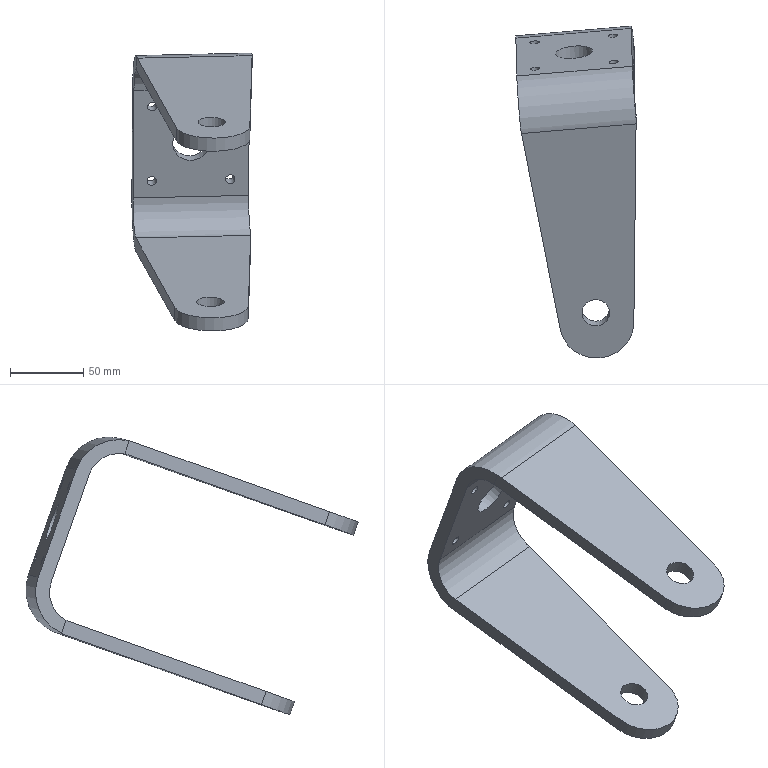Part | NX | features solid 2 | 1 solid | 25 faces | box 82.324 x 227.523 x 190.251 mm | volume 304271 mm3 | cylinder 13 | plane 12 | commonest cylinder face diameters 6.35 x4 19 x2 42.95 x2 50.8 x2 62 x2 25.4 x1
STEP:
#1=CARTESIAN_POINT('',(180.018,413.948,712.362));
#2=VERTEX_POINT('',#1);
#3=CARTESIAN_POINT('',(179.425,439.961,638.776));
#4=VERTEX_POINT('',#3);
#5=CARTESIAN_POINT('',(180.016,414.039,712.102));
#6=DIRECTION('',(0.007596,-0.3333,0.9428));
#7=VECTOR('',#6,1000.);
#8=LINE('',#5,#7);
#9=EDGE_CURVE('',#2,#4,#8,.F.);
#10=ORIENTED_EDGE('',*,*,#9,.T.);
#11=CARTESIAN_POINT('',(100.353,433.263,637.046));
#12=VERTEX_POINT('',#11);
#13=CARTESIAN_POINT('',(100.353,433.263,637.046));
#14=DIRECTION('',(0.9962,0.08438,0.0218));
#15=VECTOR('',#14,1000.);
#16=LINE('',#13,#15);
#17=EDGE_CURVE('',#4,#12,#16,.F.);
#18=ORIENTED_EDGE('',*,*,#17,.T.);
#19=CARTESIAN_POINT('',(100.945,407.25,710.631));
#20=VERTEX_POINT('',#19);
#21=CARTESIAN_POINT('',(100.354,433.179,637.281));
#22=DIRECTION('',(0.007596,-0.3333,0.9428));
#23=VECTOR('',#22,1000.);
#24=LINE('',#21,#23);
#25=EDGE_CURVE('',#12,#20,#24,.T.);
#26=ORIENTED_EDGE('',*,*,#25,.T.);
#27=CARTESIAN_POINT('',(100.945,407.25,710.631));
#28=DIRECTION('',(0.9962,0.08438,0.0218));
#29=VECTOR('',#28,1000.);
#30=LINE('',#27,#29);
#31=EDGE_CURVE('',#20,#2,#30,.T.);
#32=ORIENTED_EDGE('',*,*,#31,.T.);
#33=EDGE_LOOP('',(#10,#18,#26,#32));
#34=FACE_BOUND('',#33,.T.);
#35=CARTESIAN_POINT('',(166.841,435.935,646.855));
#36=VERTEX_POINT('',#35);
#37=CARTESIAN_POINT('',(166.865,434.877,649.848));
#38=DIRECTION('',(-0.08682,0.939,0.3327));
#39=DIRECTION('',(-0.007596,0.3333,-0.9428));
#40=AXIS2_PLACEMENT_3D('',#37,#38,#39);
#41=CIRCLE('',#40,3.175);
#42=EDGE_CURVE('',#36,#36,#41,.T.);
#43=ORIENTED_EDGE('',*,*,#42,.F.);
#44=EDGE_LOOP('',(#43));
#45=FACE_BOUND('',#44,.T.);
#46=CARTESIAN_POINT('',(113.482,413.391,696.565));
#47=VERTEX_POINT('',#46);
#48=CARTESIAN_POINT('',(113.506,412.333,699.559));
#49=DIRECTION('',(-0.08682,0.939,0.3327));
#50=DIRECTION('',(-0.007596,0.3333,-0.9428));
#51=AXIS2_PLACEMENT_3D('',#48,#49,#50);
#52=CIRCLE('',#51,3.175);
#53=EDGE_CURVE('',#47,#47,#52,.T.);
#54=ORIENTED_EDGE('',*,*,#53,.F.);
#55=EDGE_LOOP('',(#54));
#56=FACE_BOUND('',#55,.T.);
#57=CARTESIAN_POINT('',(167.251,417.946,697.742));
#58=VERTEX_POINT('',#57);
#59=CARTESIAN_POINT('',(167.275,416.888,700.736));
#60=DIRECTION('',(-0.08682,0.939,0.3327));
#61=DIRECTION('',(-0.007596,0.3333,-0.9428));
#62=AXIS2_PLACEMENT_3D('',#59,#60,#61);
#63=CIRCLE('',#62,3.175);
#64=EDGE_CURVE('',#58,#58,#63,.T.);
#65=ORIENTED_EDGE('',*,*,#64,.F.);
#66=EDGE_LOOP('',(#65));
#67=FACE_BOUND('',#66,.T.);
#68=CARTESIAN_POINT('',(140.089,427.838,662.73));
#69=VERTEX_POINT('',#68);
#70=CARTESIAN_POINT('',(140.185,423.605,674.704));
#71=DIRECTION('',(-0.08682,0.939,0.3327));
#72=DIRECTION('',(-0.007596,0.3333,-0.9428));
#73=AXIS2_PLACEMENT_3D('',#70,#71,#72);
#74=CIRCLE('',#73,12.7);
#75=EDGE_CURVE('',#69,#69,#74,.T.);
#76=ORIENTED_EDGE('',*,*,#75,.F.);
#77=EDGE_LOOP('',(#76));
#78=FACE_BOUND('',#77,.T.);
#79=CARTESIAN_POINT('',(113.072,431.381,645.678));
#80=VERTEX_POINT('',#79);
#81=CARTESIAN_POINT('',(113.096,430.322,648.672));
#82=DIRECTION('',(0.08682,-0.939,-0.3327));
#83=DIRECTION('',(-0.007596,0.3333,-0.9428));
#84=AXIS2_PLACEMENT_3D('',#81,#82,#83);
#85=CIRCLE('',#84,3.175);
#86=EDGE_CURVE('',#80,#80,#85,.T.);
#87=ORIENTED_EDGE('',*,*,#86,.T.);
#88=EDGE_LOOP('',(#87));
#89=FACE_BOUND('',#88,.T.);
#90=CARTESIAN_POINT('',(100.943,407.341,710.372));
#91=DIRECTION('',(-0.08682,0.939,0.3327));
#92=DIRECTION('',(0.9962,0.08438,0.0218));
#93=AXIS2_PLACEMENT_3D('',#90,#91,#92);
#94=PLANE('',#93);
#95=ADVANCED_FACE('',(#34,#45,#56,#67,#78,#89),#94,.T.);
#96=CARTESIAN_POINT('',(101.18,424.318,633.877));
#97=VERTEX_POINT('',#96);
#98=CARTESIAN_POINT('',(101.772,398.305,707.462));
#99=VERTEX_POINT('',#98);
#100=CARTESIAN_POINT('',(101.77,398.397,707.203));
#101=DIRECTION('',(0.007596,-0.3333,0.9428));
#102=VECTOR('',#101,1000.);
#103=LINE('',#100,#102);
#104=EDGE_CURVE('',#97,#99,#103,.T.);
#105=ORIENTED_EDGE('',*,*,#104,.F.);
#106=CARTESIAN_POINT('',(180.252,431.016,635.608));
#107=VERTEX_POINT('',#106);
#108=CARTESIAN_POINT('',(180.252,431.016,635.608));
#109=DIRECTION('',(0.9962,0.08438,0.0218));
#110=VECTOR('',#109,1000.);
#111=LINE('',#108,#110);
#112=EDGE_CURVE('',#97,#107,#111,.T.);
#113=ORIENTED_EDGE('',*,*,#112,.T.);
#114=CARTESIAN_POINT('',(180.845,405.003,709.193));
#115=VERTEX_POINT('',#114);
#116=CARTESIAN_POINT('',(180.843,405.095,708.934));
#117=DIRECTION('',(0.007596,-0.3333,0.9428));
#118=VECTOR('',#117,1000.);
#119=LINE('',#116,#118);
#120=EDGE_CURVE('',#115,#107,#119,.F.);
#121=ORIENTED_EDGE('',*,*,#120,.F.);
#122=CARTESIAN_POINT('',(101.772,398.305,707.462));
#123=DIRECTION('',(0.9962,0.08438,0.0218));
#124=VECTOR('',#123,1000.);
#125=LINE('',#122,#124);
#126=EDGE_CURVE('',#115,#99,#125,.F.);
#127=ORIENTED_EDGE('',*,*,#126,.T.);
#128=EDGE_LOOP('',(#105,#113,#121,#127));
#129=FACE_BOUND('',#128,.T.);
#130=CARTESIAN_POINT('',(167.692,424.873,649.673));
#131=VERTEX_POINT('',#130);
#132=CARTESIAN_POINT('',(167.692,425.933,646.68));
#133=DIRECTION('',(-0.08682,0.939,0.3327));
#134=DIRECTION('',(0.,-0.3339,0.9426));
#135=AXIS2_PLACEMENT_3D('',#132,#133,#134);
#136=CIRCLE('',#135,3.175);
#137=EDGE_CURVE('',#131,#131,#136,.T.);
#138=ORIENTED_EDGE('',*,*,#137,.T.);
#139=EDGE_LOOP('',(#138));
#140=FACE_BOUND('',#139,.T.);
#141=CARTESIAN_POINT('',(114.333,402.329,699.383));
#142=VERTEX_POINT('',#141);
#143=CARTESIAN_POINT('',(114.333,403.389,696.39));
#144=DIRECTION('',(-0.08682,0.939,0.3327));
#145=DIRECTION('',(0.,-0.3339,0.9426));
#146=AXIS2_PLACEMENT_3D('',#143,#144,#145);
#147=CIRCLE('',#146,3.175);
#148=EDGE_CURVE('',#142,#142,#147,.T.);
#149=ORIENTED_EDGE('',*,*,#148,.T.);
#150=EDGE_LOOP('',(#149));
#151=FACE_BOUND('',#150,.T.);
#152=CARTESIAN_POINT('',(168.102,406.883,700.56));
#153=VERTEX_POINT('',#152);
#154=CARTESIAN_POINT('',(168.102,407.944,697.567));
#155=DIRECTION('',(-0.08682,0.939,0.3327));
#156=DIRECTION('',(0.,-0.3339,0.9426));
#157=AXIS2_PLACEMENT_3D('',#154,#155,#156);
#158=CIRCLE('',#157,3.175);
#159=EDGE_CURVE('',#153,#153,#158,.T.);
#160=ORIENTED_EDGE('',*,*,#159,.T.);
#161=EDGE_LOOP('',(#160));
#162=FACE_BOUND('',#161,.T.);
#163=CARTESIAN_POINT('',(141.012,410.42,683.506));
#164=VERTEX_POINT('',#163);
#165=CARTESIAN_POINT('',(141.012,414.661,671.535));
#166=DIRECTION('',(-0.08682,0.939,0.3327));
#167=DIRECTION('',(0.,-0.3339,0.9426));
#168=AXIS2_PLACEMENT_3D('',#165,#166,#167);
#169=CIRCLE('',#168,12.7);
#170=EDGE_CURVE('',#164,#164,#169,.T.);
#171=ORIENTED_EDGE('',*,*,#170,.T.);
#172=EDGE_LOOP('',(#171));
#173=FACE_BOUND('',#172,.T.);
#174=CARTESIAN_POINT('',(113.923,420.318,648.496));
#175=VERTEX_POINT('',#174);
#176=CARTESIAN_POINT('',(113.923,421.378,645.503));
#177=DIRECTION('',(-0.08682,0.939,0.3327));
#178=DIRECTION('',(0.,-0.3339,0.9426));
#179=AXIS2_PLACEMENT_3D('',#176,#177,#178);
#180=CIRCLE('',#179,3.175);
#181=EDGE_CURVE('',#175,#175,#180,.F.);
#182=ORIENTED_EDGE('',*,*,#181,.F.);
#183=EDGE_LOOP('',(#182));
#184=FACE_BOUND('',#183,.T.);
#185=CARTESIAN_POINT('',(101.77,398.397,707.203));
#186=DIRECTION('',(-0.08682,0.939,0.3327));
#187=DIRECTION('',(0.9962,0.08438,0.0218));
#188=AXIS2_PLACEMENT_3D('',#185,#186,#187);
#189=PLANE('',#188);
#190=ADVANCED_FACE('',(#129,#140,#151,#162,#173,#184),#189,.F.);
#191=ORIENTED_EDGE('',*,*,#25,.F.);
#192=CARTESIAN_POINT('',(102.532,417.433,598.727));
#193=VERTEX_POINT('',#192);
#194=CARTESIAN_POINT('',(103.044,404.153,626.733));
#195=DIRECTION('',(-0.9962,-0.08438,-0.0218));
#196=DIRECTION('',(0.0844,-0.9964,0.));
#197=AXIS2_PLACEMENT_3D('',#194,#195,#196);
#198=CIRCLE('',#197,31.);
#199=EDGE_CURVE('',#12,#193,#198,.T.);
#200=ORIENTED_EDGE('',*,*,#199,.T.);
#201=CARTESIAN_POINT('',(102.605,414.234,607.777));
#202=VERTEX_POINT('',#201);
#203=CARTESIAN_POINT('',(102.563,416.072,602.578));
#204=DIRECTION('',(0.007596,-0.3333,0.9428));
#205=VECTOR('',#204,1000.);
#206=LINE('',#203,#205);
#207=EDGE_CURVE('',#193,#202,#206,.T.);
#208=ORIENTED_EDGE('',*,*,#207,.T.);
#209=CARTESIAN_POINT('',(103.044,404.153,626.733));
#210=DIRECTION('',(-0.9962,-0.08438,-0.0218));
#211=DIRECTION('',(0.0844,-0.9964,0.));
#212=AXIS2_PLACEMENT_3D('',#209,#210,#211);
#213=CIRCLE('',#212,21.475);
#214=EDGE_CURVE('',#202,#97,#213,.F.);
#215=ORIENTED_EDGE('',*,*,#214,.T.);
#216=ORIENTED_EDGE('',*,*,#104,.T.);
#217=CARTESIAN_POINT('',(103.521,374.065,721.403));
#218=VERTEX_POINT('',#217);
#219=CARTESIAN_POINT('',(103.637,378.139,700.318));
#220=DIRECTION('',(-0.9962,-0.08438,-0.0218));
#221=DIRECTION('',(0.0844,-0.9964,0.));
#222=AXIS2_PLACEMENT_3D('',#219,#220,#221);
#223=CIRCLE('',#222,21.475);
#224=EDGE_CURVE('',#99,#218,#223,.F.);
#225=ORIENTED_EDGE('',*,*,#224,.T.);
#226=CARTESIAN_POINT('',(103.593,370.866,730.453));
#227=VERTEX_POINT('',#226);
#228=CARTESIAN_POINT('',(102.563,416.072,602.578));
#229=DIRECTION('',(0.007596,-0.3333,0.9428));
#230=VECTOR('',#229,1000.);
#231=LINE('',#228,#230);
#232=EDGE_CURVE('',#218,#227,#231,.T.);
#233=ORIENTED_EDGE('',*,*,#232,.T.);
#234=CARTESIAN_POINT('',(103.637,378.139,700.318));
#235=DIRECTION('',(-0.9962,-0.08438,-0.0218));
#236=DIRECTION('',(0.0844,-0.9964,0.));
#237=AXIS2_PLACEMENT_3D('',#234,#235,#236);
#238=CIRCLE('',#237,31.);
#239=EDGE_CURVE('',#227,#20,#238,.T.);
#240=ORIENTED_EDGE('',*,*,#239,.T.);
#241=EDGE_LOOP('',(#191,#200,#208,#215,#216,#225,#233,#240));
#242=FACE_BOUND('',#241,.T.);
#243=CARTESIAN_POINT('',(116.683,263.361,548.479));
#244=DIRECTION('',(-0.9962,-0.08438,-0.0218));
#245=DIRECTION('',(-0.08682,0.939,0.3327));
#246=AXIS2_PLACEMENT_3D('',#243,#244,#245);
#247=PLANE('',#246);
#248=ADVANCED_FACE('',(#242),#247,.T.);
#249=CARTESIAN_POINT('',(181.678,420.932,609.507));
#250=VERTEX_POINT('',#249);
#251=CARTESIAN_POINT('',(181.605,424.131,600.457));
#252=VERTEX_POINT('',#251);
#253=CARTESIAN_POINT('',(182.635,378.926,728.333));
#254=DIRECTION('',(0.007596,-0.3333,0.9428));
#255=VECTOR('',#254,1000.);
#256=LINE('',#253,#255);
#257=EDGE_CURVE('',#250,#252,#256,.F.);
#258=ORIENTED_EDGE('',*,*,#257,.T.);
#259=CARTESIAN_POINT('',(182.117,410.851,628.464));
#260=DIRECTION('',(-0.9962,-0.08438,-0.0218));
#261=DIRECTION('',(0.0844,-0.9964,0.));
#262=AXIS2_PLACEMENT_3D('',#259,#260,#261);
#263=CIRCLE('',#262,31.);
#264=EDGE_CURVE('',#252,#4,#263,.F.);
#265=ORIENTED_EDGE('',*,*,#264,.T.);
#266=ORIENTED_EDGE('',*,*,#9,.F.);
#267=CARTESIAN_POINT('',(182.666,377.564,732.184));
#268=VERTEX_POINT('',#267);
#269=CARTESIAN_POINT('',(182.71,384.837,702.049));
#270=DIRECTION('',(-0.9962,-0.08438,-0.0218));
#271=DIRECTION('',(0.0844,-0.9964,0.));
#272=AXIS2_PLACEMENT_3D('',#269,#270,#271);
#273=CIRCLE('',#272,31.);
#274=EDGE_CURVE('',#2,#268,#273,.F.);
#275=ORIENTED_EDGE('',*,*,#274,.T.);
#276=CARTESIAN_POINT('',(182.594,380.763,723.134));
#277=VERTEX_POINT('',#276);
#278=CARTESIAN_POINT('',(182.635,378.926,728.333));
#279=DIRECTION('',(0.007596,-0.3333,0.9428));
#280=VECTOR('',#279,1000.);
#281=LINE('',#278,#280);
#282=EDGE_CURVE('',#268,#277,#281,.F.);
#283=ORIENTED_EDGE('',*,*,#282,.T.);
#284=CARTESIAN_POINT('',(182.71,384.837,702.049));
#285=DIRECTION('',(-0.9962,-0.08438,-0.0218));
#286=DIRECTION('',(0.0844,-0.9964,0.));
#287=AXIS2_PLACEMENT_3D('',#284,#285,#286);
#288=CIRCLE('',#287,21.475);
#289=EDGE_CURVE('',#277,#115,#288,.T.);
#290=ORIENTED_EDGE('',*,*,#289,.T.);
#291=ORIENTED_EDGE('',*,*,#120,.T.);
#292=CARTESIAN_POINT('',(182.117,410.851,628.464));
#293=DIRECTION('',(-0.9962,-0.08438,-0.0218));
#294=DIRECTION('',(0.0844,-0.9964,0.));
#295=AXIS2_PLACEMENT_3D('',#292,#293,#294);
#296=CIRCLE('',#295,21.475);
#297=EDGE_CURVE('',#107,#250,#296,.T.);
#298=ORIENTED_EDGE('',*,*,#297,.T.);
#299=EDGE_LOOP('',(#258,#265,#266,#275,#283,#290,#291,#298));
#300=FACE_BOUND('',#299,.T.);
#301=CARTESIAN_POINT('',(194.774,247.641,681.824));
#302=DIRECTION('',(-0.9962,-0.08438,-0.0218));
#303=DIRECTION('',(0.08682,-0.939,-0.3327));
#304=AXIS2_PLACEMENT_3D('',#301,#302,#303);
#305=PLANE('',#304);
#306=ADVANCED_FACE('',(#300),#305,.F.);
#307=CARTESIAN_POINT('',(104.112,371.008,720.572));
#308=VERTEX_POINT('',#307);
#309=CARTESIAN_POINT('',(130.665,236.884,672.943));
#310=VERTEX_POINT('',#309);
#311=CARTESIAN_POINT('',(129.04,245.088,675.856));
#312=DIRECTION('',(0.1834,-0.9264,-0.329));
#313=VECTOR('',#312,1000.);
#314=LINE('',#311,#313);
#315=EDGE_CURVE('',#308,#310,#314,.T.);
#316=ORIENTED_EDGE('',*,*,#315,.F.);
#317=CARTESIAN_POINT('',(182.561,377.654,722.289));
#318=VERTEX_POINT('',#317);
#319=CARTESIAN_POINT('',(182.873,377.68,722.296));
#320=DIRECTION('',(0.9962,0.08438,0.0218));
#321=VECTOR('',#320,1000.);
#322=LINE('',#319,#321);
#323=EDGE_CURVE('',#308,#318,#322,.T.);
#324=ORIENTED_EDGE('',*,*,#323,.T.);
#325=CARTESIAN_POINT('',(181.031,241.15,674.046));
#326=VERTEX_POINT('',#325);
#327=CARTESIAN_POINT('',(181.043,242.215,674.422));
#328=DIRECTION('',(0.01057,0.9428,0.3332));
#329=VECTOR('',#328,1000.);
#330=LINE('',#327,#329);
#331=EDGE_CURVE('',#326,#318,#330,.T.);
#332=ORIENTED_EDGE('',*,*,#331,.F.);
#333=CARTESIAN_POINT('',(155.633,241.339,674.317));
#334=DIRECTION('',(0.007596,-0.3333,0.9428));
#335=DIRECTION('',(0.,-0.9428,-0.3333));
#336=AXIS2_PLACEMENT_3D('',#333,#334,#335);
#337=CIRCLE('',#336,25.4);
#338=EDGE_CURVE('',#310,#326,#337,.T.);
#339=ORIENTED_EDGE('',*,*,#338,.F.);
#340=EDGE_LOOP('',(#316,#324,#332,#339));
#341=FACE_BOUND('',#340,.T.);
#342=CARTESIAN_POINT('',(154.98,239.449,673.654));
#343=VERTEX_POINT('',#342);
#344=CARTESIAN_POINT('',(154.98,248.406,676.82));
#345=DIRECTION('',(0.007596,-0.3333,0.9428));
#346=DIRECTION('',(0.,-0.9428,-0.3333));
#347=AXIS2_PLACEMENT_3D('',#344,#345,#346);
#348=CIRCLE('',#347,9.5);
#349=EDGE_CURVE('',#343,#343,#348,.T.);
#350=ORIENTED_EDGE('',*,*,#349,.T.);
#351=EDGE_LOOP('',(#350));
#352=FACE_BOUND('',#351,.T.);
#353=CARTESIAN_POINT('',(115.661,242.701,675.12));
#354=DIRECTION('',(0.007596,-0.3333,0.9428));
#355=DIRECTION('',(0.9962,0.08438,0.0218));
#356=AXIS2_PLACEMENT_3D('',#353,#354,#355);
#357=PLANE('',#356);
#358=ADVANCED_FACE('',(#341,#352),#357,.F.);
#359=CARTESIAN_POINT('',(181.642,417.981,608.211));
#360=VERTEX_POINT('',#359);
#361=CARTESIAN_POINT('',(180.112,281.478,559.968));
#362=VERTEX_POINT('',#361);
#363=CARTESIAN_POINT('',(181.603,414.455,606.964));
#364=DIRECTION('',(-0.01057,-0.9428,-0.3332));
#365=VECTOR('',#364,1000.);
#366=LINE('',#363,#365);
#367=EDGE_CURVE('',#360,#362,#366,.T.);
#368=ORIENTED_EDGE('',*,*,#367,.F.);
#369=CARTESIAN_POINT('',(103.193,411.336,606.494));
#370=VERTEX_POINT('',#369);
#371=CARTESIAN_POINT('',(102.881,411.31,606.487));
#372=DIRECTION('',(0.9962,0.08438,0.0218));
#373=VECTOR('',#372,1000.);
#374=LINE('',#371,#373);
#375=EDGE_CURVE('',#360,#370,#374,.F.);
#376=ORIENTED_EDGE('',*,*,#375,.T.);
#377=CARTESIAN_POINT('',(129.745,277.212,558.865));
#378=VERTEX_POINT('',#377);
#379=CARTESIAN_POINT('',(102.462,415.029,607.805));
#380=DIRECTION('',(-0.1834,0.9264,0.329));
#381=VECTOR('',#380,1000.);
#382=LINE('',#379,#381);
#383=EDGE_CURVE('',#378,#370,#382,.T.);
#384=ORIENTED_EDGE('',*,*,#383,.F.);
#385=CARTESIAN_POINT('',(154.714,281.667,560.239));
#386=DIRECTION('',(-0.007596,0.3333,-0.9428));
#387=DIRECTION('',(0.,0.9428,0.3333));
#388=AXIS2_PLACEMENT_3D('',#385,#386,#387);
#389=CIRCLE('',#388,25.4);
#390=EDGE_CURVE('',#362,#378,#389,.T.);
#391=ORIENTED_EDGE('',*,*,#390,.F.);
#392=EDGE_LOOP('',(#368,#376,#384,#391));
#393=FACE_BOUND('',#392,.T.);
#394=CARTESIAN_POINT('',(154.061,297.69,565.909));
#395=VERTEX_POINT('',#394);
#396=CARTESIAN_POINT('',(154.061,288.733,562.742));
#397=DIRECTION('',(-0.007596,0.3333,-0.9428));
#398=DIRECTION('',(0.,0.9428,0.3333));
#399=AXIS2_PLACEMENT_3D('',#396,#397,#398);
#400=CIRCLE('',#399,9.5);
#401=EDGE_CURVE('',#395,#395,#400,.T.);
#402=ORIENTED_EDGE('',*,*,#401,.T.);
#403=EDGE_LOOP('',(#402));
#404=FACE_BOUND('',#403,.T.);
#405=CARTESIAN_POINT('',(102.536,415.043,607.809));
#406=DIRECTION('',(-0.007596,0.3333,-0.9428));
#407=DIRECTION('',(-0.9962,-0.08438,-0.0218));
#408=AXIS2_PLACEMENT_3D('',#405,#406,#407);
#409=PLANE('',#408);
#410=ADVANCED_FACE('',(#393,#404),#409,.F.);
#411=CARTESIAN_POINT('',(155.052,236.274,682.634));
#412=VERTEX_POINT('',#411);
#413=CARTESIAN_POINT('',(155.052,245.231,685.8));
#414=DIRECTION('',(0.007596,-0.3333,0.9428));
#415=DIRECTION('',(0.,-0.9428,-0.3333));
#416=AXIS2_PLACEMENT_3D('',#413,#414,#415);
#417=CIRCLE('',#416,9.5);
#418=EDGE_CURVE('',#412,#412,#417,.T.);
#419=ORIENTED_EDGE('',*,*,#418,.F.);
#420=EDGE_LOOP('',(#419));
#421=FACE_BOUND('',#420,.T.);
#422=CARTESIAN_POINT('',(181.103,237.976,683.026));
#423=VERTEX_POINT('',#422);
#424=CARTESIAN_POINT('',(182.634,374.479,731.269));
#425=VERTEX_POINT('',#424);
#426=CARTESIAN_POINT('',(181.115,239.04,683.402));
#427=DIRECTION('',(0.01057,0.9428,0.3332));
#428=VECTOR('',#427,1000.);
#429=LINE('',#426,#428);
#430=EDGE_CURVE('',#423,#425,#429,.T.);
#431=ORIENTED_EDGE('',*,*,#430,.T.);
#432=CARTESIAN_POINT('',(104.184,367.834,729.552));
#433=VERTEX_POINT('',#432);
#434=CARTESIAN_POINT('',(103.872,367.807,729.545));
#435=DIRECTION('',(0.9962,0.08438,0.0218));
#436=VECTOR('',#435,1000.);
#437=LINE('',#434,#436);
#438=EDGE_CURVE('',#425,#433,#437,.F.);
#439=ORIENTED_EDGE('',*,*,#438,.T.);
#440=CARTESIAN_POINT('',(130.737,233.709,681.923));
#441=VERTEX_POINT('',#440);
#442=CARTESIAN_POINT('',(129.113,241.913,684.837));
#443=DIRECTION('',(0.1834,-0.9264,-0.329));
#444=VECTOR('',#443,1000.);
#445=LINE('',#442,#444);
#446=EDGE_CURVE('',#433,#441,#445,.T.);
#447=ORIENTED_EDGE('',*,*,#446,.T.);
#448=CARTESIAN_POINT('',(155.705,238.165,683.297));
#449=DIRECTION('',(0.007596,-0.3333,0.9428));
#450=DIRECTION('',(0.,-0.9428,-0.3333));
#451=AXIS2_PLACEMENT_3D('',#448,#449,#450);
#452=CIRCLE('',#451,25.4);
#453=EDGE_CURVE('',#441,#423,#452,.T.);
#454=ORIENTED_EDGE('',*,*,#453,.T.);
#455=EDGE_LOOP('',(#431,#439,#447,#454));
#456=FACE_BOUND('',#455,.T.);
#457=CARTESIAN_POINT('',(115.733,239.526,684.1));
#458=DIRECTION('',(0.007596,-0.3333,0.9428));
#459=DIRECTION('',(0.9962,0.08438,0.0218));
#460=AXIS2_PLACEMENT_3D('',#457,#458,#459);
#461=PLANE('',#460);
#462=ADVANCED_FACE('',(#421,#456),#461,.T.);
#463=CARTESIAN_POINT('',(153.988,300.865,556.928));
#464=VERTEX_POINT('',#463);
#465=CARTESIAN_POINT('',(153.988,291.908,553.762));
#466=DIRECTION('',(-0.007596,0.3333,-0.9428));
#467=DIRECTION('',(0.,0.9428,0.3333));
#468=AXIS2_PLACEMENT_3D('',#465,#466,#467);
#469=CIRCLE('',#468,9.5);
#470=EDGE_CURVE('',#464,#464,#469,.T.);
#471=ORIENTED_EDGE('',*,*,#470,.F.);
#472=EDGE_LOOP('',(#471));
#473=FACE_BOUND('',#472,.T.);
#474=CARTESIAN_POINT('',(129.673,280.387,549.885));
#475=VERTEX_POINT('',#474);
#476=CARTESIAN_POINT('',(103.12,414.511,597.513));
#477=VERTEX_POINT('',#476);
#478=CARTESIAN_POINT('',(102.389,418.204,598.825));
#479=DIRECTION('',(-0.1834,0.9264,0.329));
#480=VECTOR('',#479,1000.);
#481=LINE('',#478,#480);
#482=EDGE_CURVE('',#475,#477,#481,.T.);
#483=ORIENTED_EDGE('',*,*,#482,.T.);
#484=CARTESIAN_POINT('',(181.57,421.156,599.231));
#485=VERTEX_POINT('',#484);
#486=CARTESIAN_POINT('',(102.809,414.484,597.507));
#487=DIRECTION('',(0.9962,0.08438,0.0218));
#488=VECTOR('',#487,1000.);
#489=LINE('',#486,#488);
#490=EDGE_CURVE('',#477,#485,#489,.T.);
#491=ORIENTED_EDGE('',*,*,#490,.T.);
#492=CARTESIAN_POINT('',(180.039,284.653,550.987));
#493=VERTEX_POINT('',#492);
#494=CARTESIAN_POINT('',(181.53,417.629,597.984));
#495=DIRECTION('',(-0.01057,-0.9428,-0.3332));
#496=VECTOR('',#495,1000.);
#497=LINE('',#494,#496);
#498=EDGE_CURVE('',#485,#493,#497,.T.);
#499=ORIENTED_EDGE('',*,*,#498,.T.);
#500=CARTESIAN_POINT('',(154.642,284.842,551.259));
#501=DIRECTION('',(-0.007596,0.3333,-0.9428));
#502=DIRECTION('',(0.,0.9428,0.3333));
#503=AXIS2_PLACEMENT_3D('',#500,#501,#502);
#504=CIRCLE('',#503,25.4);
#505=EDGE_CURVE('',#493,#475,#504,.T.);
#506=ORIENTED_EDGE('',*,*,#505,.T.);
#507=EDGE_LOOP('',(#483,#491,#499,#506));
#508=FACE_BOUND('',#507,.T.);
#509=CARTESIAN_POINT('',(102.463,418.217,598.829));
#510=DIRECTION('',(-0.007596,0.3333,-0.9428));
#511=DIRECTION('',(-0.9962,-0.08438,-0.0218));
#512=AXIS2_PLACEMENT_3D('',#509,#510,#511);
#513=PLANE('',#512);
#514=ADVANCED_FACE('',(#473,#508),#513,.T.);
#515=ORIENTED_EDGE('',*,*,#498,.F.);
#516=CARTESIAN_POINT('',(181.805,410.824,628.457));
#517=DIRECTION('',(0.9999,-0.007435,-0.01068));
#518=DIRECTION('',(0.01057,0.9428,0.3332));
#519=AXIS2_PLACEMENT_3D('',#516,#517,#518);
#520=ELLIPSE('',#519,31.148,31.);
#521=EDGE_CURVE('',#485,#252,#520,.T.);
#522=ORIENTED_EDGE('',*,*,#521,.T.);
#523=ORIENTED_EDGE('',*,*,#257,.F.);
#524=CARTESIAN_POINT('',(181.805,410.824,628.457));
#525=DIRECTION('',(0.9999,-0.007435,-0.01068));
#526=DIRECTION('',(-0.01057,-0.9428,-0.3332));
#527=AXIS2_PLACEMENT_3D('',#524,#525,#526);
#528=ELLIPSE('',#527,21.577,21.475);
#529=EDGE_CURVE('',#250,#360,#528,.F.);
#530=ORIENTED_EDGE('',*,*,#529,.T.);
#531=ORIENTED_EDGE('',*,*,#367,.T.);
#532=CARTESIAN_POINT('',(179.855,292.725,528.153));
#533=DIRECTION('',(-0.007596,0.3333,-0.9428));
#534=VECTOR('',#533,1000.);
#535=LINE('',#532,#534);
#536=EDGE_CURVE('',#493,#362,#535,.F.);
#537=ORIENTED_EDGE('',*,*,#536,.F.);
#538=EDGE_LOOP('',(#515,#522,#523,#530,#531,#537));
#539=FACE_BOUND('',#538,.T.);
#540=CARTESIAN_POINT('',(181.428,432.983,577.723));
#541=DIRECTION('',(0.9999,-0.007435,-0.01068));
#542=DIRECTION('',(-0.01057,-0.9428,-0.3332));
#543=AXIS2_PLACEMENT_3D('',#540,#541,#542);
#544=PLANE('',#543);
#545=ADVANCED_FACE('',(#539),#544,.T.);
#546=ORIENTED_EDGE('',*,*,#207,.F.);
#547=CARTESIAN_POINT('',(103.356,404.179,626.74));
#548=DIRECTION('',(-0.983,-0.1754,-0.05409));
#549=DIRECTION('',(0.1834,-0.9264,-0.329));
#550=AXIS2_PLACEMENT_3D('',#547,#548,#549);
#551=ELLIPSE('',#550,31.148,31.);
#552=EDGE_CURVE('',#193,#477,#551,.T.);
#553=ORIENTED_EDGE('',*,*,#552,.T.);
#554=ORIENTED_EDGE('',*,*,#482,.F.);
#555=CARTESIAN_POINT('',(129.489,288.459,527.051));
#556=DIRECTION('',(0.007596,-0.3333,0.9428));
#557=VECTOR('',#556,1000.);
#558=LINE('',#555,#557);
#559=EDGE_CURVE('',#475,#378,#558,.T.);
#560=ORIENTED_EDGE('',*,*,#559,.T.);
#561=ORIENTED_EDGE('',*,*,#383,.T.);
#562=CARTESIAN_POINT('',(103.356,404.179,626.74));
#563=DIRECTION('',(-0.983,-0.1754,-0.05409));
#564=DIRECTION('',(-0.1834,0.9264,0.329));
#565=AXIS2_PLACEMENT_3D('',#562,#563,#564);
#566=ELLIPSE('',#565,21.577,21.475);
#567=EDGE_CURVE('',#370,#202,#566,.F.);
#568=ORIENTED_EDGE('',*,*,#567,.T.);
#569=EDGE_LOOP('',(#546,#553,#554,#560,#561,#568));
#570=FACE_BOUND('',#569,.T.);
#571=CARTESIAN_POINT('',(102.206,426.272,575.989));
#572=DIRECTION('',(-0.983,-0.1754,-0.05409));
#573=DIRECTION('',(-0.1834,0.9264,0.329));
#574=AXIS2_PLACEMENT_3D('',#571,#572,#573);
#575=PLANE('',#574);
#576=ADVANCED_FACE('',(#570),#575,.T.);
#577=ORIENTED_EDGE('',*,*,#390,.T.);
#578=ORIENTED_EDGE('',*,*,#559,.F.);
#579=ORIENTED_EDGE('',*,*,#505,.F.);
#580=ORIENTED_EDGE('',*,*,#536,.T.);
#581=EDGE_LOOP('',(#577,#578,#579,#580));
#582=FACE_BOUND('',#581,.T.);
#583=CARTESIAN_POINT('',(154.458,292.914,528.424));
#584=DIRECTION('',(0.007596,-0.3333,0.9428));
#585=DIRECTION('',(0.,-0.9428,-0.3333));
#586=AXIS2_PLACEMENT_3D('',#583,#584,#585);
#587=CYLINDRICAL_SURFACE('',#586,25.4);
#588=ADVANCED_FACE('',(#582),#587,.T.);
#589=ORIENTED_EDGE('',*,*,#338,.T.);
#590=CARTESIAN_POINT('',(179.855,292.725,528.153));
#591=DIRECTION('',(0.007596,-0.3333,0.9428));
#592=VECTOR('',#591,1000.);
#593=LINE('',#590,#592);
#594=EDGE_CURVE('',#326,#423,#593,.T.);
#595=ORIENTED_EDGE('',*,*,#594,.T.);
#596=ORIENTED_EDGE('',*,*,#453,.F.);
#597=CARTESIAN_POINT('',(129.489,288.459,527.051));
#598=DIRECTION('',(-0.007596,0.3333,-0.9428));
#599=VECTOR('',#598,1000.);
#600=LINE('',#597,#599);
#601=EDGE_CURVE('',#310,#441,#600,.F.);
#602=ORIENTED_EDGE('',*,*,#601,.F.);
#603=EDGE_LOOP('',(#589,#595,#596,#602));
#604=FACE_BOUND('',#603,.T.);
#605=CARTESIAN_POINT('',(154.458,292.914,528.424));
#606=DIRECTION('',(-0.007596,0.3333,-0.9428));
#607=DIRECTION('',(0.,0.9428,0.3333));
#608=AXIS2_PLACEMENT_3D('',#605,#606,#607);
#609=CYLINDRICAL_SURFACE('',#608,25.4);
#610=ADVANCED_FACE('',(#604),#609,.T.);
#611=ORIENTED_EDGE('',*,*,#282,.F.);
#612=CARTESIAN_POINT('',(182.398,384.811,702.042));
#613=DIRECTION('',(0.9999,-0.007435,-0.01068));
#614=DIRECTION('',(0.01057,0.9428,0.3332));
#615=AXIS2_PLACEMENT_3D('',#612,#613,#614);
#616=ELLIPSE('',#615,31.148,31.);
#617=EDGE_CURVE('',#268,#425,#616,.T.);
#618=ORIENTED_EDGE('',*,*,#617,.T.);
#619=ORIENTED_EDGE('',*,*,#430,.F.);
#620=ORIENTED_EDGE('',*,*,#594,.F.);
#621=ORIENTED_EDGE('',*,*,#331,.T.);
#622=CARTESIAN_POINT('',(182.398,384.811,702.042));
#623=DIRECTION('',(0.9999,-0.007435,-0.01068));
#624=DIRECTION('',(-0.01057,-0.9428,-0.3332));
#625=AXIS2_PLACEMENT_3D('',#622,#623,#624);
#626=ELLIPSE('',#625,21.577,21.475);
#627=EDGE_CURVE('',#318,#277,#626,.F.);
#628=ORIENTED_EDGE('',*,*,#627,.T.);
#629=EDGE_LOOP('',(#611,#618,#619,#620,#621,#628));
#630=FACE_BOUND('',#629,.T.);
#631=CARTESIAN_POINT('',(181.428,432.983,577.723));
#632=DIRECTION('',(0.9999,-0.007435,-0.01068));
#633=DIRECTION('',(-0.01057,-0.9428,-0.3332));
#634=AXIS2_PLACEMENT_3D('',#631,#632,#633);
#635=PLANE('',#634);
#636=ADVANCED_FACE('',(#630),#635,.T.);
#637=ORIENTED_EDGE('',*,*,#446,.F.);
#638=CARTESIAN_POINT('',(103.949,378.166,700.325));
#639=DIRECTION('',(-0.983,-0.1754,-0.05409));
#640=DIRECTION('',(0.1834,-0.9264,-0.329));
#641=AXIS2_PLACEMENT_3D('',#638,#639,#640);
#642=ELLIPSE('',#641,31.148,31.);
#643=EDGE_CURVE('',#433,#227,#642,.T.);
#644=ORIENTED_EDGE('',*,*,#643,.T.);
#645=ORIENTED_EDGE('',*,*,#232,.F.);
#646=CARTESIAN_POINT('',(103.949,378.166,700.325));
#647=DIRECTION('',(-0.983,-0.1754,-0.05409));
#648=DIRECTION('',(-0.1834,0.9264,0.329));
#649=AXIS2_PLACEMENT_3D('',#646,#647,#648);
#650=ELLIPSE('',#649,21.577,21.475);
#651=EDGE_CURVE('',#218,#308,#650,.F.);
#652=ORIENTED_EDGE('',*,*,#651,.T.);
#653=ORIENTED_EDGE('',*,*,#315,.T.);
#654=ORIENTED_EDGE('',*,*,#601,.T.);
#655=EDGE_LOOP('',(#637,#644,#645,#652,#653,#654));
#656=FACE_BOUND('',#655,.T.);
#657=CARTESIAN_POINT('',(102.206,426.272,575.989));
#658=DIRECTION('',(-0.983,-0.1754,-0.05409));
#659=DIRECTION('',(-0.1834,0.9264,0.329));
#660=AXIS2_PLACEMENT_3D('',#657,#658,#659);
#661=PLANE('',#660);
#662=ADVANCED_FACE('',(#656),#661,.T.);
#663=ORIENTED_EDGE('',*,*,#470,.T.);
#664=EDGE_LOOP('',(#663));
#665=FACE_BOUND('',#664,.T.);
#666=ORIENTED_EDGE('',*,*,#401,.F.);
#667=EDGE_LOOP('',(#666));
#668=FACE_BOUND('',#667,.T.);
#669=CARTESIAN_POINT('',(153.187,327.07,454.297));
#670=DIRECTION('',(0.007596,-0.3333,0.9428));
#671=DIRECTION('',(0.9962,0.08438,0.0218));
#672=AXIS2_PLACEMENT_3D('',#669,#670,#671);
#673=CYLINDRICAL_SURFACE('',#672,9.5);
#674=ADVANCED_FACE('',(#665,#668),#673,.F.);
#675=ORIENTED_EDGE('',*,*,#418,.T.);
#676=EDGE_LOOP('',(#675));
#677=FACE_BOUND('',#676,.T.);
#678=ORIENTED_EDGE('',*,*,#349,.F.);
#679=EDGE_LOOP('',(#678));
#680=FACE_BOUND('',#679,.T.);
#681=CARTESIAN_POINT('',(153.187,327.07,454.297));
#682=DIRECTION('',(0.007596,-0.3333,0.9428));
#683=DIRECTION('',(0.9962,0.08438,0.0218));
#684=AXIS2_PLACEMENT_3D('',#681,#682,#683);
#685=CYLINDRICAL_SURFACE('',#684,9.5);
#686=ADVANCED_FACE('',(#677,#680),#685,.F.);
#687=ORIENTED_EDGE('',*,*,#42,.T.);
#688=EDGE_LOOP('',(#687));
#689=FACE_BOUND('',#688,.T.);
#690=ORIENTED_EDGE('',*,*,#137,.F.);
#691=EDGE_LOOP('',(#690));
#692=FACE_BOUND('',#691,.T.);
#693=CARTESIAN_POINT('',(171.717,382.404,631.259));
#694=DIRECTION('',(-0.08682,0.939,0.3327));
#695=DIRECTION('',(0.9962,0.08438,0.0218));
#696=AXIS2_PLACEMENT_3D('',#693,#694,#695);
#697=CYLINDRICAL_SURFACE('',#696,3.175);
#698=ADVANCED_FACE('',(#689,#692),#697,.F.);
#699=ORIENTED_EDGE('',*,*,#53,.T.);
#700=EDGE_LOOP('',(#699));
#701=FACE_BOUND('',#700,.T.);
#702=ORIENTED_EDGE('',*,*,#148,.F.);
#703=EDGE_LOOP('',(#702));
#704=FACE_BOUND('',#703,.T.);
#705=CARTESIAN_POINT('',(118.357,359.86,680.97));
#706=DIRECTION('',(-0.08682,0.939,0.3327));
#707=DIRECTION('',(0.9962,0.08438,0.0218));
#708=AXIS2_PLACEMENT_3D('',#705,#706,#707);
#709=CYLINDRICAL_SURFACE('',#708,3.175);
#710=ADVANCED_FACE('',(#701,#704),#709,.F.);
#711=ORIENTED_EDGE('',*,*,#64,.T.);
#712=EDGE_LOOP('',(#711));
#713=FACE_BOUND('',#712,.T.);
#714=ORIENTED_EDGE('',*,*,#159,.F.);
#715=EDGE_LOOP('',(#714));
#716=FACE_BOUND('',#715,.T.);
#717=CARTESIAN_POINT('',(172.127,364.414,682.147));
#718=DIRECTION('',(-0.08682,0.939,0.3327));
#719=DIRECTION('',(0.9962,0.08438,0.0218));
#720=AXIS2_PLACEMENT_3D('',#717,#718,#719);
#721=CYLINDRICAL_SURFACE('',#720,3.175);
#722=ADVANCED_FACE('',(#713,#716),#721,.F.);
#723=ORIENTED_EDGE('',*,*,#75,.T.);
#724=EDGE_LOOP('',(#723));
#725=FACE_BOUND('',#724,.T.);
#726=ORIENTED_EDGE('',*,*,#170,.F.);
#727=EDGE_LOOP('',(#726));
#728=FACE_BOUND('',#727,.T.);
#729=CARTESIAN_POINT('',(145.037,371.132,656.115));
#730=DIRECTION('',(-0.08682,0.939,0.3327));
#731=DIRECTION('',(0.9962,0.08438,0.0218));
#732=AXIS2_PLACEMENT_3D('',#729,#730,#731);
#733=CYLINDRICAL_SURFACE('',#732,12.7);
#734=ADVANCED_FACE('',(#725,#728),#733,.F.);
#735=ORIENTED_EDGE('',*,*,#86,.F.);
#736=EDGE_LOOP('',(#735));
#737=FACE_BOUND('',#736,.T.);
#738=ORIENTED_EDGE('',*,*,#181,.T.);
#739=EDGE_LOOP('',(#738));
#740=FACE_BOUND('',#739,.T.);
#741=CARTESIAN_POINT('',(117.947,377.849,630.082));
#742=DIRECTION('',(-0.08682,0.939,0.3327));
#743=DIRECTION('',(0.9962,0.08438,0.0218));
#744=AXIS2_PLACEMENT_3D('',#741,#742,#743);
#745=CYLINDRICAL_SURFACE('',#744,3.175);
#746=ADVANCED_FACE('',(#737,#740),#745,.F.);
#747=ORIENTED_EDGE('',*,*,#199,.F.);
#748=ORIENTED_EDGE('',*,*,#17,.F.);
#749=ORIENTED_EDGE('',*,*,#264,.F.);
#750=ORIENTED_EDGE('',*,*,#521,.F.);
#751=ORIENTED_EDGE('',*,*,#490,.F.);
#752=ORIENTED_EDGE('',*,*,#552,.F.);
#753=EDGE_LOOP('',(#747,#748,#749,#750,#751,#752));
#754=FACE_BOUND('',#753,.T.);
#755=CARTESIAN_POINT('',(103.044,404.153,626.733));
#756=DIRECTION('',(0.9962,0.08438,0.0218));
#757=DIRECTION('',(-0.0844,0.9964,0.));
#758=AXIS2_PLACEMENT_3D('',#755,#756,#757);
#759=CYLINDRICAL_SURFACE('',#758,31.);
#760=ADVANCED_FACE('',(#754),#759,.T.);
#761=ORIENTED_EDGE('',*,*,#643,.F.);
#762=ORIENTED_EDGE('',*,*,#438,.F.);
#763=ORIENTED_EDGE('',*,*,#617,.F.);
#764=ORIENTED_EDGE('',*,*,#274,.F.);
#765=ORIENTED_EDGE('',*,*,#31,.F.);
#766=ORIENTED_EDGE('',*,*,#239,.F.);
#767=EDGE_LOOP('',(#761,#762,#763,#764,#765,#766));
#768=FACE_BOUND('',#767,.T.);
#769=CARTESIAN_POINT('',(103.637,378.139,700.318));
#770=DIRECTION('',(0.9962,0.08438,0.0218));
#771=DIRECTION('',(-0.0844,0.9964,0.));
#772=AXIS2_PLACEMENT_3D('',#769,#770,#771);
#773=CYLINDRICAL_SURFACE('',#772,31.);
#774=ADVANCED_FACE('',(#768),#773,.T.);
#775=ORIENTED_EDGE('',*,*,#567,.F.);
#776=ORIENTED_EDGE('',*,*,#375,.F.);
#777=ORIENTED_EDGE('',*,*,#529,.F.);
#778=ORIENTED_EDGE('',*,*,#297,.F.);
#779=ORIENTED_EDGE('',*,*,#112,.F.);
#780=ORIENTED_EDGE('',*,*,#214,.F.);
#781=EDGE_LOOP('',(#775,#776,#777,#778,#779,#780));
#782=FACE_BOUND('',#781,.T.);
#783=CARTESIAN_POINT('',(103.044,404.153,626.733));
#784=DIRECTION('',(-0.9962,-0.08438,-0.0218));
#785=DIRECTION('',(0.0844,-0.9964,0.));
#786=AXIS2_PLACEMENT_3D('',#783,#784,#785);
#787=CYLINDRICAL_SURFACE('',#786,21.475);
#788=ADVANCED_FACE('',(#782),#787,.F.);
#789=ORIENTED_EDGE('',*,*,#224,.F.);
#790=ORIENTED_EDGE('',*,*,#126,.F.);
#791=ORIENTED_EDGE('',*,*,#289,.F.);
#792=ORIENTED_EDGE('',*,*,#627,.F.);
#793=ORIENTED_EDGE('',*,*,#323,.F.);
#794=ORIENTED_EDGE('',*,*,#651,.F.);
#795=EDGE_LOOP('',(#789,#790,#791,#792,#793,#794));
#796=FACE_BOUND('',#795,.T.);
#797=CARTESIAN_POINT('',(103.637,378.139,700.318));
#798=DIRECTION('',(-0.9962,-0.08438,-0.0218));
#799=DIRECTION('',(0.0844,-0.9964,0.));
#800=AXIS2_PLACEMENT_3D('',#797,#798,#799);
#801=CYLINDRICAL_SURFACE('',#800,21.475);
#802=ADVANCED_FACE('',(#796),#801,.F.);
#803=CLOSED_SHELL('',(#95,#190,#248,#306,#358,#410,#462,#514,#545,#576,#588,#610,#636,#662,#674,#686,#698,#710,#722,#734,#746,#760,#774,#788,#802));
#804=MANIFOLD_SOLID_BREP('',#803);
#805=(LENGTH_UNIT()NAMED_UNIT(*)SI_UNIT(.MILLI.,.METRE.));
#806=UNCERTAINTY_MEASURE_WITH_UNIT(LENGTH_MEASURE(0.00001),#805,'','');
#807=(NAMED_UNIT(*)PLANE_ANGLE_UNIT()SI_UNIT($,.RADIAN.));
#808=(NAMED_UNIT(*)SI_UNIT($,.STERADIAN.)SOLID_ANGLE_UNIT());
#809=(GEOMETRIC_REPRESENTATION_CONTEXT(3)GLOBAL_UNCERTAINTY_ASSIGNED_CONTEXT((#806))GLOBAL_UNIT_ASSIGNED_CONTEXT((#805,#807,#808))REPRESENTATION_CONTEXT('',''));
#810=ADVANCED_BREP_SHAPE_REPRESENTATION('',(#804),#809);